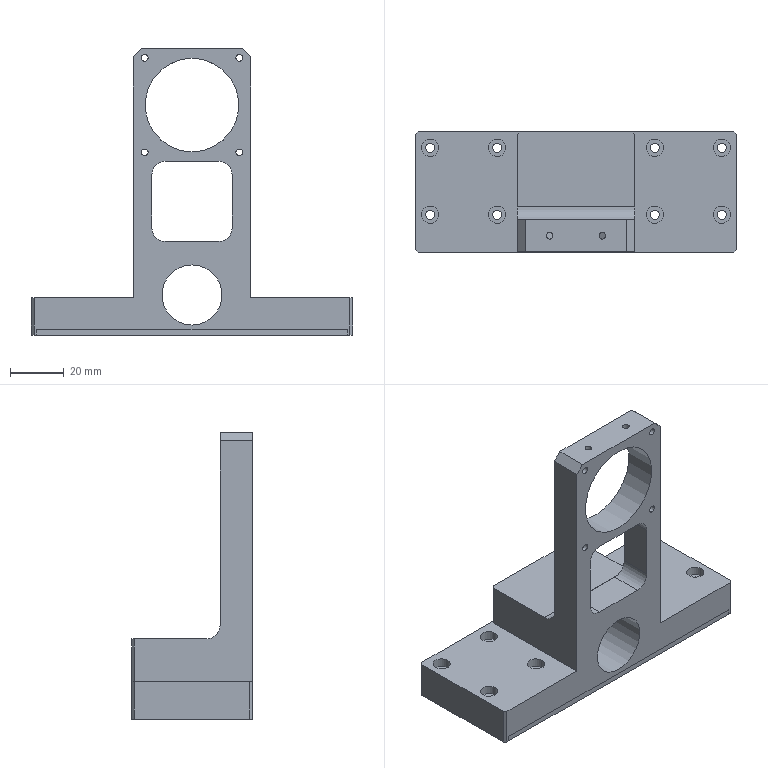CAM job | NX | 3+2 milling, drilling | part box 120 x 45 x 107 mm | stock box 125 x 50 x 110 mm
Tools:
number,name,description,diameter,corner_radius,flute_length,length,flutes
9,D10,平底铣刀-粗,10.0,0.0,35.0,75.0,2
7,D6-J,平底铣刀-精,6.0,0.0,25.0,75.0,2
10,D10-J,平底铣刀-精,10.0,0.0,35.0,75.0,2
1,D80R0.8飞刀,圆鼻刀-粗,80.0,0.8,50.0,75.0,2
2,D6倒角刀,倒角刀,6.0,0.0,3.0,25.0,2
20,M3X0.5,丝锥,2.5,0.0,35.0,50.0,2
21,M4X0.7,丝锥,3.3,0.0,35.0,50.0,2
12,ZT2.6,钻头,2.6,0.0,35.0,50.0,2
13,ZT3.4,钻头,3.4,0.0,35.0,50.0,2
17,ZT12,钻头,12.0,0.0,35.0,50.0,2
11,D4-EXTENDED-J,平底铣刀-粗,4.0,0.0,50.0,75.0,2
Operations:
program,operation,operation_type,tool,method,geometry_group,spindle_rpm,surface_speed,feed_per_tooth,feed_cut,feed_plunge,cut_length_mm,path_length_mm,cut_time_min,machine_time_min
C,打点,Operation,D6倒角刀,METHOD,W-C,3000.0,56.549,0.0333,200.0,0.0,20.0,356.128,0.1,0.1336
C,打孔,Operation,ZT3.4,METHOD,W-C,3000.0,32.044,0.0167,100.0,0.0,136.0,588.128,1.36,1.405
C,底壁铣分层开粗-中_COPY,VolumeBased25DMillingOperation,D10,分层开粗-切深K-步距G,W-C,8000.0,251.32,0.25,4000.0,100.0,4188.228,4289.13,1.047,1.057
C,底壁铣精光底面-中_COPY_2,VolumeBased25DMillingOperation,D10-J,精光步距切深关,W-C,8000.0,251.32,0.0625,1000.0,100.0,1140.639,1162.439,1.141,1.143
C,NG_钻倒角_4,Operation,D6倒角刀,METHOD,W-C,5000.0,94.248,0.015,150.0,0.0,40.0,415.152,0.2667,0.3042
C,平面去毛刺6X45L_COPY_2,SurfaceContour,D6倒角刀,爬面_倒角-切深0-步距G,W-C,6500.0,122.519,0.1154,1500.0,100.0,489.932,1351.55,0.3266,0.4128
C,底壁铣精光侧面-中-选底面_COPY_1,VolumeBased25DMillingOperation,D10-J,侧刃精光-切深K-步距G,W-C,8000.0,251.327,0.05,800.0,100.0,126.386,250.542,0.158,0.1704
B,动态开粗D10_COPY_1,CavityMilling,D10,动态开粗-切深K-步距K,W-B,8000.0,251.32,0.25,4000.0,100.0,17854.396,17950.196,4.464,4.473
B,底壁铣精光底面-中_COPY,VolumeBased25DMillingOperation,D10-J,精光步距切深关,W-B,7000.0,175.0,0.0536,1500.0,100.0,687.639,713.639,0.4584,0.461
B,动态开粗D10_COPY_2,CavityMilling,D10,动态开粗-切深K-步距K,W-B,8000.0,251.32,0.25,4000.0,100.0,13885.074,15732.67,3.471,3.656
B,打点-深0.8_2,Operation,D6倒角刀,NONE,W-B,8000.0,150.796,0.0312,500.0,90.0,14.4,389.855,0.0288,0.0663
B,NG_盲锥孔-M4螺纹底孔,Operation,ZT3.4,NONE,W-B,3000.0,31.102,0.02,120.0,90.0,52.0,264.93,0.4333,0.4546
B,NG_钻倒角_2,Operation,D6倒角刀,METHOD,W-B,8000.0,150.796,0.0312,500.0,0.0,19.0,319.447,0.038,0.068
B,NG_钻倒角_3,Operation,D6倒角刀,METHOD,W-B,8000.0,150.796,0.0312,500.0,0.0,20.8,209.189,0.0416,0.0604
B,平面去毛刺6X45L_COPY,SurfaceContour,D6倒角刀,爬面_倒角-切深0-步距G,W-B,6500.0,122.519,0.1154,1500.0,100.0,745.752,1564.035,0.4972,0.579
B,底壁铣倒角_COPY_1,VolumeBased25DMillingOperation,D6倒角刀,爬面_倒角-切深0-步距G,W-B,6500.0,122.519,0.1154,1500.0,100.0,45.601,367.817,0.0304,0.0626
B,平面去毛刺6X45L_COPY_1,SurfaceContour,D6倒角刀,爬面_倒角-切深0-步距G,W-B,6500.0,122.519,0.1154,1500.0,100.0,261.752,363.474,0.1745,0.1847
B,盲锥孔-攻牙M4,Operation,M4X0.7,METHOD,W-B,800.0,8.294,0.0004,0.7,90.0,36.4,233.73,52.0,52.02
B,底壁铣精光底面-中_COPY_1,VolumeBased25DMillingOperation,D10-J,精光步距切深关,W-B,7000.0,175.0,0.0536,1500.0,100.0,611.064,703.064,0.4074,0.4166
B,底壁铣精光侧面-中-选底面_COPY,VolumeBased25DMillingOperation,D10-J,侧刃精光-切深K-步距G,W-B,8000.0,251.32,0.0625,1000.0,100.0,51.365,160.365,0.0514,0.0623
B,底壁铣精光侧面-中_COPY_2,VolumeBased25DMillingOperation,D10-J,侧刃精光-切深K-步距G,W-B,8000.0,251.32,0.0625,1000.0,100.0,186.152,365.016,0.1862,0.204
B,等高精光往复爬面_COPY,ZLevelMilling,D10-J,等高爬面-切深K-步距G,W-B,7000.0,219.911,0.25,3500.0,100.0,22597.92,22687.435,6.457,6.465
A,顶面,FaceMilling,D80R0.8飞刀,侧刃精光-切深K-步距G,W-A,4500.0,1385.0,0.1667,1500.0,100.0,707.5,803.5,0.4717,0.4813
A,动态开粗D10_COPY,CavityMilling,D10,动态开粗-切深K-步距K,W-A,8000.0,251.32,0.25,4000.0,100.0,39256.431,40145.057,9.814,9.903
A,打点-深0.8,Operation,D6倒角刀,NONE,W-A,8000.0,150.796,0.0312,500.0,90.0,10.8,303.564,0.0216,0.0509
A,通孔-M3螺纹底孔,Operation,ZT2.6,NONE,W-A,3000.0,23.562,0.05,300.0,90.0,76.0,361.108,0.2533,0.2818
A,NG_钻倒角_1,Operation,D6倒角刀,METHOD,W-A,8000.0,150.796,0.0312,500.0,0.0,19.0,253.447,0.038,0.0614
A,通孔-攻牙M3,Operation,M3X0.5,METHOD,W-A,800.0,6.283,0.0003,0.5,90.0,64.0,337.108,128.0,128.027
A,通孔-12.5-25,Operation,ZT12,NONE,W-A,800.0,30.159,0.125,200.0,90.0,51.605,203.21,0.258,0.2732
A,通孔-精孔12.0预钻,Operation,ZT12,NONE,W-A,800.0,87.462,0.125,200.0,90.0,18.105,136.21,0.0905,0.1023
A,框开粗_1,VolumeBased25DMillingOperation,D10,METHOD,W-A,9000.0,169.646,0.1111,2000.0,80.0,2219.14,2330.14,1.11,1.121
A,铣孔开粗D8_1,CylinderMilling,D10,NONE,W-A,8000.0,251.327,0.125,2000.0,100.0,3613.286,3758.286,1.807,1.821
A,铣孔开粗D8_2,CylinderMilling,D10,NONE,W-A,8000.0,251.327,0.125,2000.0,100.0,3621.819,3759.819,1.811,1.825
A,框精_1,VolumeBased25DMillingOperation,D6-J,METHOD,W-A,8000.0,100.531,0.0625,1000.0,100.0,195.444,432.26,0.1954,0.2191
A,等高光顺清角D4参考10_COPY,ZLevelMilling,D4-EXTENDED-J,分层精光-切深K-步距G,W-A,8000.0,100.531,0.125,2000.0,100.0,3815.395,4153.097,1.908,1.942
A,底壁铣精光侧面-中_COPY,VolumeBased25DMillingOperation,D10-J,侧刃精光-切深K-步距G,W-A,8000.0,251.32,0.0625,1000.0,100.0,241.342,351.65,0.2413,0.2524
A,外形半精_2,VolumeBased25DMillingOperation,D10-J,METHOD,W-A,9000.0,169.646,0.0667,1200.0,100.0,1930.269,2558.813,1.609,1.671
A,仅选体,SurfaceContour,D6倒角刀,METHOD,W-A,8000.0,150.796,0.1875,3000.0,100.0,732.078,1381.977,0.244,0.309
A,铣倒角_1,PlanarMilling,D6倒角刀,METHOD,W-A,8000.0,150.796,0.0625,1000.0,100.0,73.571,175.571,0.0736,0.0838
A,铣倒角_2,PlanarMilling,D6倒角刀,METHOD,W-A,8000.0,150.796,0.0312,500.0,100.0,115.982,216.982,0.232,0.2421
A,底壁铣倒角_COPY,VolumeBased25DMillingOperation,D6倒角刀,爬面_倒角-切深0-步距G,W-A,6500.0,122.519,0.1154,1500.0,100.0,45.601,367.817,0.0304,0.0626
A,底壁铣精光侧面-中_COPY_1,VolumeBased25DMillingOperation,D10-J,侧刃精光-切深K-步距G,W-A,8000.0,251.327,0.05,800.0,100.0,174.891,217.759,0.2186,0.2229